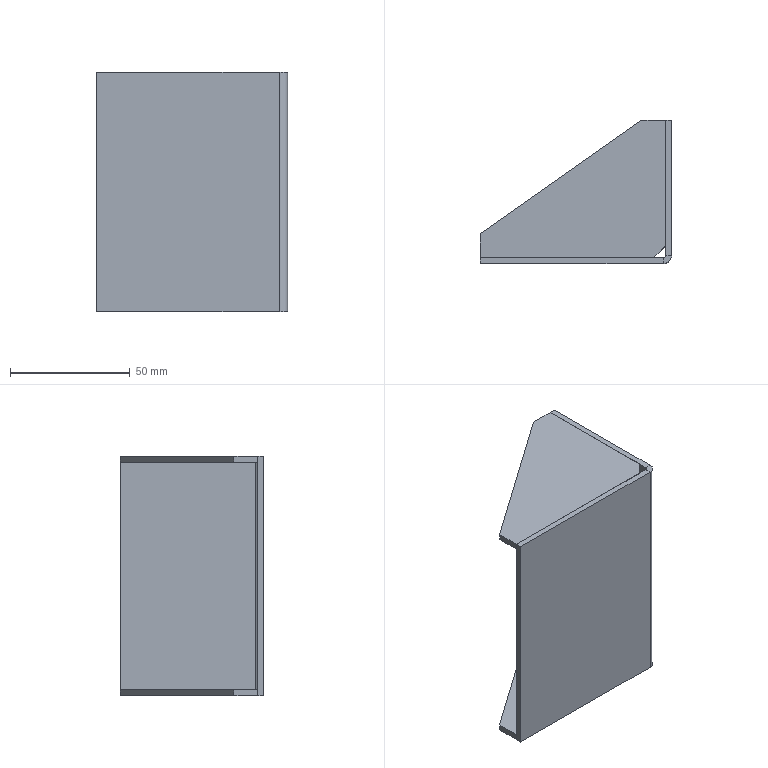Part | SolidWorks | features BaseBody 3 | 3 solids | 30 faces | box 80 x 60 x 100 mm | volume 48337 mm3 | plane 28 | cylinder 2 | commonest cylinder face diameters 2 x1 7 x1
STEP:
#1=CARTESIAN_POINT('',(-3.5,-57.5,-50.));
#2=VERTEX_POINT('',#1);
#3=CARTESIAN_POINT('',(-80.,-57.5,-50.));
#4=VERTEX_POINT('',#3);
#5=CARTESIAN_POINT('',(0.,-57.5,-50.));
#6=DIRECTION('',(-1.,0.,0.));
#7=VECTOR('',#6,1000.);
#8=LINE('',#5,#7);
#9=EDGE_CURVE('',#2,#4,#8,.T.);
#10=ORIENTED_EDGE('',*,*,#9,.F.);
#11=CARTESIAN_POINT('',(-3.5,-60.,-50.));
#12=VERTEX_POINT('',#11);
#13=CARTESIAN_POINT('',(-3.5,-57.5,-50.));
#14=DIRECTION('',(0.,-1.,0.));
#15=VECTOR('',#14,1000.);
#16=LINE('',#13,#15);
#17=EDGE_CURVE('',#2,#12,#16,.T.);
#18=ORIENTED_EDGE('',*,*,#17,.T.);
#19=CARTESIAN_POINT('',(-80.,-60.,-50.));
#20=VERTEX_POINT('',#19);
#21=CARTESIAN_POINT('',(0.,-60.,-50.));
#22=DIRECTION('',(-1.,0.,0.));
#23=VECTOR('',#22,1000.);
#24=LINE('',#21,#23);
#25=EDGE_CURVE('',#12,#20,#24,.T.);
#26=ORIENTED_EDGE('',*,*,#25,.T.);
#27=CARTESIAN_POINT('',(-80.,-60.,-50.));
#28=DIRECTION('',(0.,1.,0.));
#29=VECTOR('',#28,1000.);
#30=LINE('',#27,#29);
#31=EDGE_CURVE('',#20,#4,#30,.T.);
#32=ORIENTED_EDGE('',*,*,#31,.T.);
#33=EDGE_LOOP('',(#10,#18,#26,#32));
#34=FACE_OUTER_BOUND('',#33,.T.);
#35=CARTESIAN_POINT('',(-3.5,-56.5,-50.));
#36=DIRECTION('',(0.,0.,1.));
#37=DIRECTION('',(1.,0.,0.));
#38=AXIS2_PLACEMENT_3D('',#35,#36,#37);
#39=PLANE('',#38);
#40=ADVANCED_FACE('',(#34),#39,.F.);
#41=CARTESIAN_POINT('',(-2.5,0.,50.));
#42=VERTEX_POINT('',#41);
#43=CARTESIAN_POINT('',(-2.5,-56.5,50.));
#44=VERTEX_POINT('',#43);
#45=CARTESIAN_POINT('',(-2.5,0.,50.));
#46=DIRECTION('',(0.,-1.,0.));
#47=VECTOR('',#46,1000.);
#48=LINE('',#45,#47);
#49=EDGE_CURVE('',#42,#44,#48,.T.);
#50=ORIENTED_EDGE('',*,*,#49,.T.);
#51=CARTESIAN_POINT('',(0.,-56.5,50.));
#52=VERTEX_POINT('',#51);
#53=CARTESIAN_POINT('',(-2.5,-56.5,50.));
#54=DIRECTION('',(1.,0.,0.));
#55=VECTOR('',#54,1000.);
#56=LINE('',#53,#55);
#57=EDGE_CURVE('',#44,#52,#56,.T.);
#58=ORIENTED_EDGE('',*,*,#57,.T.);
#59=CARTESIAN_POINT('',(0.,0.,50.));
#60=VERTEX_POINT('',#59);
#61=CARTESIAN_POINT('',(0.,0.,50.));
#62=DIRECTION('',(0.,-1.,0.));
#63=VECTOR('',#62,1000.);
#64=LINE('',#61,#63);
#65=EDGE_CURVE('',#60,#52,#64,.T.);
#66=ORIENTED_EDGE('',*,*,#65,.F.);
#67=CARTESIAN_POINT('',(-2.5,0.,50.));
#68=DIRECTION('',(1.,0.,0.));
#69=VECTOR('',#68,1000.);
#70=LINE('',#67,#69);
#71=EDGE_CURVE('',#42,#60,#70,.T.);
#72=ORIENTED_EDGE('',*,*,#71,.F.);
#73=EDGE_LOOP('',(#50,#58,#66,#72));
#74=FACE_OUTER_BOUND('',#73,.T.);
#75=CARTESIAN_POINT('',(-3.5,-56.5,50.));
#76=DIRECTION('',(0.,0.,1.));
#77=DIRECTION('',(1.,0.,0.));
#78=AXIS2_PLACEMENT_3D('',#75,#76,#77);
#79=PLANE('',#78);
#80=ADVANCED_FACE('',(#74),#79,.T.);
#81=CARTESIAN_POINT('',(-2.5,-56.5,-50.));
#82=VERTEX_POINT('',#81);
#83=CARTESIAN_POINT('',(-3.5,-56.5,-50.));
#84=DIRECTION('',(0.,0.,-1.));
#85=DIRECTION('',(1.,0.,0.));
#86=AXIS2_PLACEMENT_3D('',#83,#84,#85);
#87=CIRCLE('',#86,1.);
#88=EDGE_CURVE('',#82,#2,#87,.T.);
#89=ORIENTED_EDGE('',*,*,#88,.T.);
#90=CARTESIAN_POINT('',(-3.5,-57.5,50.));
#91=VERTEX_POINT('',#90);
#92=CARTESIAN_POINT('',(-3.5,-57.5,50.));
#93=DIRECTION('',(0.,0.,-1.));
#94=VECTOR('',#93,1000.);
#95=LINE('',#92,#94);
#96=EDGE_CURVE('',#91,#2,#95,.T.);
#97=ORIENTED_EDGE('',*,*,#96,.F.);
#98=CARTESIAN_POINT('',(-3.5,-56.5,50.));
#99=DIRECTION('',(0.,0.,-1.));
#100=DIRECTION('',(1.,0.,0.));
#101=AXIS2_PLACEMENT_3D('',#98,#99,#100);
#102=CIRCLE('',#101,1.);
#103=EDGE_CURVE('',#44,#91,#102,.T.);
#104=ORIENTED_EDGE('',*,*,#103,.F.);
#105=CARTESIAN_POINT('',(-2.5,-56.5,50.));
#106=DIRECTION('',(0.,0.,-1.));
#107=VECTOR('',#106,1000.);
#108=LINE('',#105,#107);
#109=EDGE_CURVE('',#44,#82,#108,.T.);
#110=ORIENTED_EDGE('',*,*,#109,.T.);
#111=EDGE_LOOP('',(#89,#97,#104,#110));
#112=FACE_OUTER_BOUND('',#111,.T.);
#113=CARTESIAN_POINT('',(-3.5,-56.5,50.));
#114=DIRECTION('',(0.,0.,-1.));
#115=DIRECTION('',(-1.,0.,0.));
#116=AXIS2_PLACEMENT_3D('',#113,#114,#115);
#117=CYLINDRICAL_SURFACE('',#116,1.);
#118=ADVANCED_FACE('',(#112),#117,.F.);
#119=CARTESIAN_POINT('',(-2.5,0.,-50.));
#120=VERTEX_POINT('',#119);
#121=CARTESIAN_POINT('',(-2.5,0.,-50.));
#122=DIRECTION('',(0.,-1.,0.));
#123=VECTOR('',#122,1000.);
#124=LINE('',#121,#123);
#125=EDGE_CURVE('',#120,#82,#124,.T.);
#126=ORIENTED_EDGE('',*,*,#125,.T.);
#127=ORIENTED_EDGE('',*,*,#109,.F.);
#128=ORIENTED_EDGE('',*,*,#49,.F.);
#129=CARTESIAN_POINT('',(-2.5,0.,50.));
#130=DIRECTION('',(0.,0.,-1.));
#131=VECTOR('',#130,1000.);
#132=LINE('',#129,#131);
#133=EDGE_CURVE('',#42,#120,#132,.T.);
#134=ORIENTED_EDGE('',*,*,#133,.T.);
#135=EDGE_LOOP('',(#126,#127,#128,#134));
#136=FACE_OUTER_BOUND('',#135,.T.);
#137=CARTESIAN_POINT('',(-2.5,0.,50.));
#138=DIRECTION('',(1.,0.,0.));
#139=DIRECTION('',(0.,1.,0.));
#140=AXIS2_PLACEMENT_3D('',#137,#138,#139);
#141=PLANE('',#140);
#142=ADVANCED_FACE('',(#136),#141,.F.);
#143=CARTESIAN_POINT('',(0.,0.,-50.));
#144=VERTEX_POINT('',#143);
#145=CARTESIAN_POINT('',(-2.5,0.,-50.));
#146=DIRECTION('',(1.,0.,0.));
#147=VECTOR('',#146,1000.);
#148=LINE('',#145,#147);
#149=EDGE_CURVE('',#120,#144,#148,.T.);
#150=ORIENTED_EDGE('',*,*,#149,.F.);
#151=ORIENTED_EDGE('',*,*,#133,.F.);
#152=ORIENTED_EDGE('',*,*,#71,.T.);
#153=CARTESIAN_POINT('',(0.,0.,50.));
#154=DIRECTION('',(0.,0.,-1.));
#155=VECTOR('',#154,1000.);
#156=LINE('',#153,#155);
#157=EDGE_CURVE('',#60,#144,#156,.T.);
#158=ORIENTED_EDGE('',*,*,#157,.T.);
#159=EDGE_LOOP('',(#150,#151,#152,#158));
#160=FACE_OUTER_BOUND('',#159,.T.);
#161=CARTESIAN_POINT('',(-2.5,0.,50.));
#162=DIRECTION('',(0.,1.,0.));
#163=DIRECTION('',(1.,0.,0.));
#164=AXIS2_PLACEMENT_3D('',#161,#162,#163);
#165=PLANE('',#164);
#166=ADVANCED_FACE('',(#160),#165,.T.);
#167=CARTESIAN_POINT('',(0.,-56.5,-50.));
#168=VERTEX_POINT('',#167);
#169=CARTESIAN_POINT('',(0.,0.,-50.));
#170=DIRECTION('',(0.,-1.,0.));
#171=VECTOR('',#170,1000.);
#172=LINE('',#169,#171);
#173=EDGE_CURVE('',#144,#168,#172,.T.);
#174=ORIENTED_EDGE('',*,*,#173,.F.);
#175=ORIENTED_EDGE('',*,*,#157,.F.);
#176=ORIENTED_EDGE('',*,*,#65,.T.);
#177=CARTESIAN_POINT('',(0.,-56.5,50.));
#178=DIRECTION('',(0.,0.,-1.));
#179=VECTOR('',#178,1000.);
#180=LINE('',#177,#179);
#181=EDGE_CURVE('',#52,#168,#180,.T.);
#182=ORIENTED_EDGE('',*,*,#181,.T.);
#183=EDGE_LOOP('',(#174,#175,#176,#182));
#184=FACE_OUTER_BOUND('',#183,.T.);
#185=CARTESIAN_POINT('',(0.,0.,50.));
#186=DIRECTION('',(1.,0.,0.));
#187=DIRECTION('',(0.,1.,0.));
#188=AXIS2_PLACEMENT_3D('',#185,#186,#187);
#189=PLANE('',#188);
#190=ADVANCED_FACE('',(#184),#189,.T.);
#191=CARTESIAN_POINT('',(-3.5,-56.5,-50.));
#192=DIRECTION('',(0.,0.,-1.));
#193=DIRECTION('',(1.,0.,0.));
#194=AXIS2_PLACEMENT_3D('',#191,#192,#193);
#195=CIRCLE('',#194,3.5);
#196=EDGE_CURVE('',#168,#12,#195,.T.);
#197=ORIENTED_EDGE('',*,*,#196,.F.);
#198=ORIENTED_EDGE('',*,*,#181,.F.);
#199=CARTESIAN_POINT('',(-3.5,-60.,50.));
#200=VERTEX_POINT('',#199);
#201=CARTESIAN_POINT('',(-3.5,-56.5,50.));
#202=DIRECTION('',(0.,0.,-1.));
#203=DIRECTION('',(1.,0.,0.));
#204=AXIS2_PLACEMENT_3D('',#201,#202,#203);
#205=CIRCLE('',#204,3.5);
#206=EDGE_CURVE('',#52,#200,#205,.T.);
#207=ORIENTED_EDGE('',*,*,#206,.T.);
#208=CARTESIAN_POINT('',(-3.5,-60.,50.));
#209=DIRECTION('',(0.,0.,-1.));
#210=VECTOR('',#209,1000.);
#211=LINE('',#208,#210);
#212=EDGE_CURVE('',#200,#12,#211,.T.);
#213=ORIENTED_EDGE('',*,*,#212,.T.);
#214=EDGE_LOOP('',(#197,#198,#207,#213));
#215=FACE_OUTER_BOUND('',#214,.T.);
#216=CARTESIAN_POINT('',(-3.5,-56.5,50.));
#217=DIRECTION('',(0.,0.,-1.));
#218=DIRECTION('',(-1.,0.,0.));
#219=AXIS2_PLACEMENT_3D('',#216,#217,#218);
#220=CYLINDRICAL_SURFACE('',#219,3.5);
#221=ADVANCED_FACE('',(#215),#220,.T.);
#222=ORIENTED_EDGE('',*,*,#25,.F.);
#223=ORIENTED_EDGE('',*,*,#212,.F.);
#224=CARTESIAN_POINT('',(-80.,-60.,50.));
#225=VERTEX_POINT('',#224);
#226=CARTESIAN_POINT('',(0.,-60.,50.));
#227=DIRECTION('',(-1.,0.,0.));
#228=VECTOR('',#227,1000.);
#229=LINE('',#226,#228);
#230=EDGE_CURVE('',#200,#225,#229,.T.);
#231=ORIENTED_EDGE('',*,*,#230,.T.);
#232=CARTESIAN_POINT('',(-80.,-60.,50.));
#233=DIRECTION('',(0.,0.,-1.));
#234=VECTOR('',#233,1000.);
#235=LINE('',#232,#234);
#236=EDGE_CURVE('',#225,#20,#235,.T.);
#237=ORIENTED_EDGE('',*,*,#236,.T.);
#238=EDGE_LOOP('',(#222,#223,#231,#237));
#239=FACE_OUTER_BOUND('',#238,.T.);
#240=CARTESIAN_POINT('',(0.,-60.,50.));
#241=DIRECTION('',(0.,-1.,0.));
#242=DIRECTION('',(0.,0.,-1.));
#243=AXIS2_PLACEMENT_3D('',#240,#241,#242);
#244=PLANE('',#243);
#245=ADVANCED_FACE('',(#239),#244,.T.);
#246=ORIENTED_EDGE('',*,*,#31,.F.);
#247=ORIENTED_EDGE('',*,*,#236,.F.);
#248=CARTESIAN_POINT('',(-80.,-57.5,50.));
#249=VERTEX_POINT('',#248);
#250=CARTESIAN_POINT('',(-80.,-60.,50.));
#251=DIRECTION('',(0.,1.,0.));
#252=VECTOR('',#251,1000.);
#253=LINE('',#250,#252);
#254=EDGE_CURVE('',#225,#249,#253,.T.);
#255=ORIENTED_EDGE('',*,*,#254,.T.);
#256=CARTESIAN_POINT('',(-80.,-57.5,50.));
#257=DIRECTION('',(0.,0.,-1.));
#258=VECTOR('',#257,1000.);
#259=LINE('',#256,#258);
#260=EDGE_CURVE('',#249,#4,#259,.T.);
#261=ORIENTED_EDGE('',*,*,#260,.T.);
#262=EDGE_LOOP('',(#246,#247,#255,#261));
#263=FACE_OUTER_BOUND('',#262,.T.);
#264=CARTESIAN_POINT('',(-80.,-60.,50.));
#265=DIRECTION('',(-1.,0.,0.));
#266=DIRECTION('',(0.,0.,1.));
#267=AXIS2_PLACEMENT_3D('',#264,#265,#266);
#268=PLANE('',#267);
#269=ADVANCED_FACE('',(#263),#268,.T.);
#270=ORIENTED_EDGE('',*,*,#9,.T.);
#271=ORIENTED_EDGE('',*,*,#260,.F.);
#272=CARTESIAN_POINT('',(0.,-57.5,50.));
#273=DIRECTION('',(-1.,0.,0.));
#274=VECTOR('',#273,1000.);
#275=LINE('',#272,#274);
#276=EDGE_CURVE('',#91,#249,#275,.T.);
#277=ORIENTED_EDGE('',*,*,#276,.F.);
#278=ORIENTED_EDGE('',*,*,#96,.T.);
#279=EDGE_LOOP('',(#270,#271,#277,#278));
#280=FACE_OUTER_BOUND('',#279,.T.);
#281=CARTESIAN_POINT('',(0.,-57.5,50.));
#282=DIRECTION('',(0.,-1.,0.));
#283=DIRECTION('',(0.,0.,-1.));
#284=AXIS2_PLACEMENT_3D('',#281,#282,#283);
#285=PLANE('',#284);
#286=ADVANCED_FACE('',(#280),#285,.F.);
#287=ORIENTED_EDGE('',*,*,#173,.T.);
#288=CARTESIAN_POINT('',(0.,-56.5,-50.));
#289=DIRECTION('',(-1.,0.,0.));
#290=VECTOR('',#289,1000.);
#291=LINE('',#288,#290);
#292=EDGE_CURVE('',#168,#82,#291,.T.);
#293=ORIENTED_EDGE('',*,*,#292,.T.);
#294=ORIENTED_EDGE('',*,*,#125,.F.);
#295=ORIENTED_EDGE('',*,*,#149,.T.);
#296=EDGE_LOOP('',(#287,#293,#294,#295));
#297=FACE_OUTER_BOUND('',#296,.T.);
#298=CARTESIAN_POINT('',(-3.5,-57.5,-50.));
#299=DIRECTION('',(0.,0.,-1.));
#300=DIRECTION('',(0.,-1.,0.));
#301=AXIS2_PLACEMENT_3D('',#298,#299,#300);
#302=PLANE('',#301);
#303=ADVANCED_FACE('',(#297),#302,.T.);
#304=ORIENTED_EDGE('',*,*,#292,.F.);
#305=ORIENTED_EDGE('',*,*,#196,.T.);
#306=ORIENTED_EDGE('',*,*,#17,.F.);
#307=ORIENTED_EDGE('',*,*,#88,.F.);
#308=EDGE_LOOP('',(#304,#305,#306,#307));
#309=FACE_OUTER_BOUND('',#308,.T.);
#310=CARTESIAN_POINT('',(0.,-56.5,-50.));
#311=DIRECTION('',(0.,0.,-1.));
#312=DIRECTION('',(0.,-1.,0.));
#313=AXIS2_PLACEMENT_3D('',#310,#311,#312);
#314=PLANE('',#313);
#315=ADVANCED_FACE('',(#309),#314,.T.);
#316=ORIENTED_EDGE('',*,*,#230,.F.);
#317=CARTESIAN_POINT('',(-3.5,-60.,50.));
#318=DIRECTION('',(0.,1.,0.));
#319=VECTOR('',#318,1000.);
#320=LINE('',#317,#319);
#321=EDGE_CURVE('',#200,#91,#320,.T.);
#322=ORIENTED_EDGE('',*,*,#321,.T.);
#323=ORIENTED_EDGE('',*,*,#276,.T.);
#324=ORIENTED_EDGE('',*,*,#254,.F.);
#325=EDGE_LOOP('',(#316,#322,#323,#324));
#326=FACE_OUTER_BOUND('',#325,.T.);
#327=CARTESIAN_POINT('',(-2.5,-56.5,50.));
#328=DIRECTION('',(0.,0.,1.));
#329=DIRECTION('',(1.,0.,0.));
#330=AXIS2_PLACEMENT_3D('',#327,#328,#329);
#331=PLANE('',#330);
#332=ADVANCED_FACE('',(#326),#331,.T.);
#333=ORIENTED_EDGE('',*,*,#321,.F.);
#334=ORIENTED_EDGE('',*,*,#206,.F.);
#335=ORIENTED_EDGE('',*,*,#57,.F.);
#336=ORIENTED_EDGE('',*,*,#103,.T.);
#337=EDGE_LOOP('',(#333,#334,#335,#336));
#338=FACE_OUTER_BOUND('',#337,.T.);
#339=CARTESIAN_POINT('',(-3.5,-60.,50.));
#340=DIRECTION('',(0.,0.,1.));
#341=DIRECTION('',(1.,0.,0.));
#342=AXIS2_PLACEMENT_3D('',#339,#340,#341);
#343=PLANE('',#342);
#344=ADVANCED_FACE('',(#338),#343,.T.);
#345=CLOSED_SHELL('',(#40,#80,#118,#142,#166,#190,#221,#245,#269,#286,#303,#315,#332,#344));
#346=MANIFOLD_SOLID_BREP('',#345);
#347=CARTESIAN_POINT('',(-2.5,0.,-50.));
#348=VERTEX_POINT('',#347);
#349=CARTESIAN_POINT('',(-2.5,-52.5,-50.));
#350=VERTEX_POINT('',#349);
#351=CARTESIAN_POINT('',(-2.5,-52.5,-50.));
#352=DIRECTION('',(0.,-1.,0.));
#353=VECTOR('',#352,1000.);
#354=LINE('',#351,#353);
#355=EDGE_CURVE('',#348,#350,#354,.T.);
#356=ORIENTED_EDGE('',*,*,#355,.T.);
#357=CARTESIAN_POINT('',(-7.5,-57.5,-50.));
#358=VERTEX_POINT('',#357);
#359=CARTESIAN_POINT('',(-7.5,-57.5,-50.));
#360=DIRECTION('',(-0.7071,-0.7071,0.));
#361=VECTOR('',#360,1000.);
#362=LINE('',#359,#361);
#363=EDGE_CURVE('',#350,#358,#362,.T.);
#364=ORIENTED_EDGE('',*,*,#363,.T.);
#365=CARTESIAN_POINT('',(-80.,-57.5,-50.));
#366=VERTEX_POINT('',#365);
#367=CARTESIAN_POINT('',(-80.,-57.5,-50.));
#368=DIRECTION('',(-1.,0.,0.));
#369=VECTOR('',#368,1000.);
#370=LINE('',#367,#369);
#371=EDGE_CURVE('',#358,#366,#370,.T.);
#372=ORIENTED_EDGE('',*,*,#371,.T.);
#373=CARTESIAN_POINT('',(-80.,-47.5,-50.));
#374=VERTEX_POINT('',#373);
#375=CARTESIAN_POINT('',(-80.,-47.5,-50.));
#376=DIRECTION('',(0.,1.,0.));
#377=VECTOR('',#376,1000.);
#378=LINE('',#375,#377);
#379=EDGE_CURVE('',#366,#374,#378,.T.);
#380=ORIENTED_EDGE('',*,*,#379,.T.);
#381=CARTESIAN_POINT('',(-12.5,0.,-50.));
#382=VERTEX_POINT('',#381);
#383=CARTESIAN_POINT('',(-12.5,0.,-50.));
#384=DIRECTION('',(0.8178,0.5755,0.));
#385=VECTOR('',#384,1000.);
#386=LINE('',#383,#385);
#387=EDGE_CURVE('',#374,#382,#386,.T.);
#388=ORIENTED_EDGE('',*,*,#387,.T.);
#389=CARTESIAN_POINT('',(-2.5,0.,-50.));
#390=DIRECTION('',(1.,0.,0.));
#391=VECTOR('',#390,1000.);
#392=LINE('',#389,#391);
#393=EDGE_CURVE('',#382,#348,#392,.T.);
#394=ORIENTED_EDGE('',*,*,#393,.T.);
#395=EDGE_LOOP('',(#356,#364,#372,#380,#388,#394));
#396=FACE_OUTER_BOUND('',#395,.T.);
#397=CARTESIAN_POINT('',(0.,0.,-50.));
#398=DIRECTION('',(0.,0.,1.));
#399=DIRECTION('',(1.,0.,0.));
#400=AXIS2_PLACEMENT_3D('',#397,#398,#399);
#401=PLANE('',#400);
#402=ADVANCED_FACE('',(#396),#401,.F.);
#403=CARTESIAN_POINT('',(-2.5,0.,-47.5));
#404=VERTEX_POINT('',#403);
#405=CARTESIAN_POINT('',(-2.5,-52.5,-47.5));
#406=VERTEX_POINT('',#405);
#407=CARTESIAN_POINT('',(-2.5,-52.5,-47.5));
#408=DIRECTION('',(0.,-1.,0.));
#409=VECTOR('',#408,1000.);
#410=LINE('',#407,#409);
#411=EDGE_CURVE('',#404,#406,#410,.T.);
#412=ORIENTED_EDGE('',*,*,#411,.F.);
#413=CARTESIAN_POINT('',(-12.5,0.,-47.5));
#414=VERTEX_POINT('',#413);
#415=CARTESIAN_POINT('',(-2.5,0.,-47.5));
#416=DIRECTION('',(1.,0.,0.));
#417=VECTOR('',#416,1000.);
#418=LINE('',#415,#417);
#419=EDGE_CURVE('',#414,#404,#418,.T.);
#420=ORIENTED_EDGE('',*,*,#419,.F.);
#421=CARTESIAN_POINT('',(-80.,-47.5,-47.5));
#422=VERTEX_POINT('',#421);
#423=CARTESIAN_POINT('',(-12.5,0.,-47.5));
#424=DIRECTION('',(0.8178,0.5755,0.));
#425=VECTOR('',#424,1000.);
#426=LINE('',#423,#425);
#427=EDGE_CURVE('',#422,#414,#426,.T.);
#428=ORIENTED_EDGE('',*,*,#427,.F.);
#429=CARTESIAN_POINT('',(-80.,-57.5,-47.5));
#430=VERTEX_POINT('',#429);
#431=CARTESIAN_POINT('',(-80.,-47.5,-47.5));
#432=DIRECTION('',(0.,1.,0.));
#433=VECTOR('',#432,1000.);
#434=LINE('',#431,#433);
#435=EDGE_CURVE('',#430,#422,#434,.T.);
#436=ORIENTED_EDGE('',*,*,#435,.F.);
#437=CARTESIAN_POINT('',(-7.5,-57.5,-47.5));
#438=VERTEX_POINT('',#437);
#439=CARTESIAN_POINT('',(-80.,-57.5,-47.5));
#440=DIRECTION('',(-1.,0.,0.));
#441=VECTOR('',#440,1000.);
#442=LINE('',#439,#441);
#443=EDGE_CURVE('',#438,#430,#442,.T.);
#444=ORIENTED_EDGE('',*,*,#443,.F.);
#445=CARTESIAN_POINT('',(-7.5,-57.5,-47.5));
#446=DIRECTION('',(-0.7071,-0.7071,0.));
#447=VECTOR('',#446,1000.);
#448=LINE('',#445,#447);
#449=EDGE_CURVE('',#406,#438,#448,.T.);
#450=ORIENTED_EDGE('',*,*,#449,.F.);
#451=EDGE_LOOP('',(#412,#420,#428,#436,#444,#450));
#452=FACE_OUTER_BOUND('',#451,.T.);
#453=CARTESIAN_POINT('',(0.,0.,-47.5));
#454=DIRECTION('',(0.,0.,1.));
#455=DIRECTION('',(1.,0.,0.));
#456=AXIS2_PLACEMENT_3D('',#453,#454,#455);
#457=PLANE('',#456);
#458=ADVANCED_FACE('',(#452),#457,.T.);
#459=ORIENTED_EDGE('',*,*,#363,.F.);
#460=CARTESIAN_POINT('',(-2.5,-52.5,-47.5));
#461=DIRECTION('',(0.,0.,-1.));
#462=VECTOR('',#461,1000.);
#463=LINE('',#460,#462);
#464=EDGE_CURVE('',#406,#350,#463,.T.);
#465=ORIENTED_EDGE('',*,*,#464,.F.);
#466=ORIENTED_EDGE('',*,*,#449,.T.);
#467=CARTESIAN_POINT('',(-7.5,-57.5,-47.5));
#468=DIRECTION('',(0.,0.,-1.));
#469=VECTOR('',#468,1000.);
#470=LINE('',#467,#469);
#471=EDGE_CURVE('',#438,#358,#470,.T.);
#472=ORIENTED_EDGE('',*,*,#471,.T.);
#473=EDGE_LOOP('',(#459,#465,#466,#472));
#474=FACE_OUTER_BOUND('',#473,.T.);
#475=CARTESIAN_POINT('',(-7.5,-57.5,-47.5));
#476=DIRECTION('',(0.7071,-0.7071,0.));
#477=DIRECTION('',(0.,0.,-1.));
#478=AXIS2_PLACEMENT_3D('',#475,#476,#477);
#479=PLANE('',#478);
#480=ADVANCED_FACE('',(#474),#479,.T.);
#481=ORIENTED_EDGE('',*,*,#371,.F.);
#482=ORIENTED_EDGE('',*,*,#471,.F.);
#483=ORIENTED_EDGE('',*,*,#443,.T.);
#484=CARTESIAN_POINT('',(-80.,-57.5,-47.5));
#485=DIRECTION('',(0.,0.,-1.));
#486=VECTOR('',#485,1000.);
#487=LINE('',#484,#486);
#488=EDGE_CURVE('',#430,#366,#487,.T.);
#489=ORIENTED_EDGE('',*,*,#488,.T.);
#490=EDGE_LOOP('',(#481,#482,#483,#489));
#491=FACE_OUTER_BOUND('',#490,.T.);
#492=CARTESIAN_POINT('',(-80.,-57.5,-47.5));
#493=DIRECTION('',(0.,-1.,0.));
#494=DIRECTION('',(-1.,0.,0.));
#495=AXIS2_PLACEMENT_3D('',#492,#493,#494);
#496=PLANE('',#495);
#497=ADVANCED_FACE('',(#491),#496,.T.);
#498=ORIENTED_EDGE('',*,*,#379,.F.);
#499=ORIENTED_EDGE('',*,*,#488,.F.);
#500=ORIENTED_EDGE('',*,*,#435,.T.);
#501=CARTESIAN_POINT('',(-80.,-47.5,-47.5));
#502=DIRECTION('',(0.,0.,-1.));
#503=VECTOR('',#502,1000.);
#504=LINE('',#501,#503);
#505=EDGE_CURVE('',#422,#374,#504,.T.);
#506=ORIENTED_EDGE('',*,*,#505,.T.);
#507=EDGE_LOOP('',(#498,#499,#500,#506));
#508=FACE_OUTER_BOUND('',#507,.T.);
#509=CARTESIAN_POINT('',(-80.,-47.5,-47.5));
#510=DIRECTION('',(-1.,0.,0.));
#511=DIRECTION('',(0.,0.,1.));
#512=AXIS2_PLACEMENT_3D('',#509,#510,#511);
#513=PLANE('',#512);
#514=ADVANCED_FACE('',(#508),#513,.T.);
#515=ORIENTED_EDGE('',*,*,#387,.F.);
#516=ORIENTED_EDGE('',*,*,#505,.F.);
#517=ORIENTED_EDGE('',*,*,#427,.T.);
#518=CARTESIAN_POINT('',(-12.5,0.,-47.5));
#519=DIRECTION('',(0.,0.,-1.));
#520=VECTOR('',#519,1000.);
#521=LINE('',#518,#520);
#522=EDGE_CURVE('',#414,#382,#521,.T.);
#523=ORIENTED_EDGE('',*,*,#522,.T.);
#524=EDGE_LOOP('',(#515,#516,#517,#523));
#525=FACE_OUTER_BOUND('',#524,.T.);
#526=CARTESIAN_POINT('',(-12.5,0.,-47.5));
#527=DIRECTION('',(-0.5755,0.8178,0.));
#528=DIRECTION('',(0.,0.,1.));
#529=AXIS2_PLACEMENT_3D('',#526,#527,#528);
#530=PLANE('',#529);
#531=ADVANCED_FACE('',(#525),#530,.T.);
#532=ORIENTED_EDGE('',*,*,#393,.F.);
#533=ORIENTED_EDGE('',*,*,#522,.F.);
#534=ORIENTED_EDGE('',*,*,#419,.T.);
#535=CARTESIAN_POINT('',(-2.5,0.,-47.5));
#536=DIRECTION('',(0.,0.,-1.));
#537=VECTOR('',#536,1000.);
#538=LINE('',#535,#537);
#539=EDGE_CURVE('',#404,#348,#538,.T.);
#540=ORIENTED_EDGE('',*,*,#539,.T.);
#541=EDGE_LOOP('',(#532,#533,#534,#540));
#542=FACE_OUTER_BOUND('',#541,.T.);
#543=CARTESIAN_POINT('',(-2.5,0.,-47.5));
#544=DIRECTION('',(0.,1.,0.));
#545=DIRECTION('',(1.,0.,0.));
#546=AXIS2_PLACEMENT_3D('',#543,#544,#545);
#547=PLANE('',#546);
#548=ADVANCED_FACE('',(#542),#547,.T.);
#549=ORIENTED_EDGE('',*,*,#355,.F.);
#550=ORIENTED_EDGE('',*,*,#539,.F.);
#551=ORIENTED_EDGE('',*,*,#411,.T.);
#552=ORIENTED_EDGE('',*,*,#464,.T.);
#553=EDGE_LOOP('',(#549,#550,#551,#552));
#554=FACE_OUTER_BOUND('',#553,.T.);
#555=CARTESIAN_POINT('',(-2.5,-52.5,-47.5));
#556=DIRECTION('',(1.,0.,0.));
#557=DIRECTION('',(0.,1.,0.));
#558=AXIS2_PLACEMENT_3D('',#555,#556,#557);
#559=PLANE('',#558);
#560=ADVANCED_FACE('',(#554),#559,.T.);
#561=CLOSED_SHELL('',(#402,#458,#480,#497,#514,#531,#548,#560));
#562=MANIFOLD_SOLID_BREP('',#561);
#563=CARTESIAN_POINT('',(-2.5,0.,50.));
#564=VERTEX_POINT('',#563);
#565=CARTESIAN_POINT('',(-2.5,-52.5,50.));
#566=VERTEX_POINT('',#565);
#567=CARTESIAN_POINT('',(-2.5,-52.5,50.));
#568=DIRECTION('',(0.,-1.,0.));
#569=VECTOR('',#568,1000.);
#570=LINE('',#567,#569);
#571=EDGE_CURVE('',#564,#566,#570,.T.);
#572=ORIENTED_EDGE('',*,*,#571,.F.);
#573=CARTESIAN_POINT('',(-12.5,0.,50.));
#574=VERTEX_POINT('',#573);
#575=CARTESIAN_POINT('',(-2.5,0.,50.));
#576=DIRECTION('',(1.,0.,0.));
#577=VECTOR('',#576,1000.);
#578=LINE('',#575,#577);
#579=EDGE_CURVE('',#574,#564,#578,.T.);
#580=ORIENTED_EDGE('',*,*,#579,.F.);
#581=CARTESIAN_POINT('',(-80.,-47.5,50.));
#582=VERTEX_POINT('',#581);
#583=CARTESIAN_POINT('',(-12.5,0.,50.));
#584=DIRECTION('',(0.8178,0.5755,0.));
#585=VECTOR('',#584,1000.);
#586=LINE('',#583,#585);
#587=EDGE_CURVE('',#582,#574,#586,.T.);
#588=ORIENTED_EDGE('',*,*,#587,.F.);
#589=CARTESIAN_POINT('',(-80.,-57.5,50.));
#590=VERTEX_POINT('',#589);
#591=CARTESIAN_POINT('',(-80.,-47.5,50.));
#592=DIRECTION('',(0.,1.,0.));
#593=VECTOR('',#592,1000.);
#594=LINE('',#591,#593);
#595=EDGE_CURVE('',#590,#582,#594,.T.);
#596=ORIENTED_EDGE('',*,*,#595,.F.);
#597=CARTESIAN_POINT('',(-7.5,-57.5,50.));
#598=VERTEX_POINT('',#597);
#599=CARTESIAN_POINT('',(-80.,-57.5,50.));
#600=DIRECTION('',(-1.,0.,0.));
#601=VECTOR('',#600,1000.);
#602=LINE('',#599,#601);
#603=EDGE_CURVE('',#598,#590,#602,.T.);
#604=ORIENTED_EDGE('',*,*,#603,.F.);
#605=CARTESIAN_POINT('',(-7.5,-57.5,50.));
#606=DIRECTION('',(-0.7071,-0.7071,0.));
#607=VECTOR('',#606,1000.);
#608=LINE('',#605,#607);
#609=EDGE_CURVE('',#566,#598,#608,.T.);
#610=ORIENTED_EDGE('',*,*,#609,.F.);
#611=EDGE_LOOP('',(#572,#580,#588,#596,#604,#610));
#612=FACE_OUTER_BOUND('',#611,.T.);
#613=CARTESIAN_POINT('',(0.,0.,50.));
#614=DIRECTION('',(0.,0.,-1.));
#615=DIRECTION('',(0.,-1.,0.));
#616=AXIS2_PLACEMENT_3D('',#613,#614,#615);
#617=PLANE('',#616);
#618=ADVANCED_FACE('',(#612),#617,.F.);
#619=CARTESIAN_POINT('',(-2.5,0.,47.5));
#620=VERTEX_POINT('',#619);
#621=CARTESIAN_POINT('',(-2.5,-52.5,47.5));
#622=VERTEX_POINT('',#621);
#623=CARTESIAN_POINT('',(-2.5,-52.5,47.5));
#624=DIRECTION('',(0.,-1.,0.));
#625=VECTOR('',#624,1000.);
#626=LINE('',#623,#625);
#627=EDGE_CURVE('',#620,#622,#626,.T.);
#628=ORIENTED_EDGE('',*,*,#627,.T.);
#629=CARTESIAN_POINT('',(-7.5,-57.5,47.5));
#630=VERTEX_POINT('',#629);
#631=CARTESIAN_POINT('',(-7.5,-57.5,47.5));
#632=DIRECTION('',(-0.7071,-0.7071,0.));
#633=VECTOR('',#632,1000.);
#634=LINE('',#631,#633);
#635=EDGE_CURVE('',#622,#630,#634,.T.);
#636=ORIENTED_EDGE('',*,*,#635,.T.);
#637=CARTESIAN_POINT('',(-80.,-57.5,47.5));
#638=VERTEX_POINT('',#637);
#639=CARTESIAN_POINT('',(-80.,-57.5,47.5));
#640=DIRECTION('',(-1.,0.,0.));
#641=VECTOR('',#640,1000.);
#642=LINE('',#639,#641);
#643=EDGE_CURVE('',#630,#638,#642,.T.);
#644=ORIENTED_EDGE('',*,*,#643,.T.);
#645=CARTESIAN_POINT('',(-80.,-47.5,47.5));
#646=VERTEX_POINT('',#645);
#647=CARTESIAN_POINT('',(-80.,-47.5,47.5));
#648=DIRECTION('',(0.,1.,0.));
#649=VECTOR('',#648,1000.);
#650=LINE('',#647,#649);
#651=EDGE_CURVE('',#638,#646,#650,.T.);
#652=ORIENTED_EDGE('',*,*,#651,.T.);
#653=CARTESIAN_POINT('',(-12.5,0.,47.5));
#654=VERTEX_POINT('',#653);
#655=CARTESIAN_POINT('',(-12.5,0.,47.5));
#656=DIRECTION('',(0.8178,0.5755,0.));
#657=VECTOR('',#656,1000.);
#658=LINE('',#655,#657);
#659=EDGE_CURVE('',#646,#654,#658,.T.);
#660=ORIENTED_EDGE('',*,*,#659,.T.);
#661=CARTESIAN_POINT('',(-2.5,0.,47.5));
#662=DIRECTION('',(1.,0.,0.));
#663=VECTOR('',#662,1000.);
#664=LINE('',#661,#663);
#665=EDGE_CURVE('',#654,#620,#664,.T.);
#666=ORIENTED_EDGE('',*,*,#665,.T.);
#667=EDGE_LOOP('',(#628,#636,#644,#652,#660,#666));
#668=FACE_OUTER_BOUND('',#667,.T.);
#669=CARTESIAN_POINT('',(0.,0.,47.5));
#670=DIRECTION('',(0.,0.,-1.));
#671=DIRECTION('',(0.,-1.,0.));
#672=AXIS2_PLACEMENT_3D('',#669,#670,#671);
#673=PLANE('',#672);
#674=ADVANCED_FACE('',(#668),#673,.T.);
#675=ORIENTED_EDGE('',*,*,#609,.T.);
#676=CARTESIAN_POINT('',(-7.5,-57.5,47.5));
#677=DIRECTION('',(0.,0.,1.));
#678=VECTOR('',#677,1000.);
#679=LINE('',#676,#678);
#680=EDGE_CURVE('',#630,#598,#679,.T.);
#681=ORIENTED_EDGE('',*,*,#680,.F.);
#682=ORIENTED_EDGE('',*,*,#635,.F.);
#683=CARTESIAN_POINT('',(-2.5,-52.5,47.5));
#684=DIRECTION('',(0.,0.,1.));
#685=VECTOR('',#684,1000.);
#686=LINE('',#683,#685);
#687=EDGE_CURVE('',#622,#566,#686,.T.);
#688=ORIENTED_EDGE('',*,*,#687,.T.);
#689=EDGE_LOOP('',(#675,#681,#682,#688));
#690=FACE_OUTER_BOUND('',#689,.T.);
#691=CARTESIAN_POINT('',(-7.5,-57.5,47.5));
#692=DIRECTION('',(0.7071,-0.7071,0.));
#693=DIRECTION('',(0.,0.,-1.));
#694=AXIS2_PLACEMENT_3D('',#691,#692,#693);
#695=PLANE('',#694);
#696=ADVANCED_FACE('',(#690),#695,.T.);
#697=ORIENTED_EDGE('',*,*,#603,.T.);
#698=CARTESIAN_POINT('',(-80.,-57.5,47.5));
#699=DIRECTION('',(0.,0.,1.));
#700=VECTOR('',#699,1000.);
#701=LINE('',#698,#700);
#702=EDGE_CURVE('',#638,#590,#701,.T.);
#703=ORIENTED_EDGE('',*,*,#702,.F.);
#704=ORIENTED_EDGE('',*,*,#643,.F.);
#705=ORIENTED_EDGE('',*,*,#680,.T.);
#706=EDGE_LOOP('',(#697,#703,#704,#705));
#707=FACE_OUTER_BOUND('',#706,.T.);
#708=CARTESIAN_POINT('',(-80.,-57.5,47.5));
#709=DIRECTION('',(0.,-1.,0.));
#710=DIRECTION('',(-1.,0.,0.));
#711=AXIS2_PLACEMENT_3D('',#708,#709,#710);
#712=PLANE('',#711);
#713=ADVANCED_FACE('',(#707),#712,.T.);
#714=ORIENTED_EDGE('',*,*,#595,.T.);
#715=CARTESIAN_POINT('',(-80.,-47.5,47.5));
#716=DIRECTION('',(0.,0.,1.));
#717=VECTOR('',#716,1000.);
#718=LINE('',#715,#717);
#719=EDGE_CURVE('',#646,#582,#718,.T.);
#720=ORIENTED_EDGE('',*,*,#719,.F.);
#721=ORIENTED_EDGE('',*,*,#651,.F.);
#722=ORIENTED_EDGE('',*,*,#702,.T.);
#723=EDGE_LOOP('',(#714,#720,#721,#722));
#724=FACE_OUTER_BOUND('',#723,.T.);
#725=CARTESIAN_POINT('',(-80.,-47.5,47.5));
#726=DIRECTION('',(-1.,0.,0.));
#727=DIRECTION('',(0.,0.,1.));
#728=AXIS2_PLACEMENT_3D('',#725,#726,#727);
#729=PLANE('',#728);
#730=ADVANCED_FACE('',(#724),#729,.T.);
#731=ORIENTED_EDGE('',*,*,#587,.T.);
#732=CARTESIAN_POINT('',(-12.5,0.,47.5));
#733=DIRECTION('',(0.,0.,1.));
#734=VECTOR('',#733,1000.);
#735=LINE('',#732,#734);
#736=EDGE_CURVE('',#654,#574,#735,.T.);
#737=ORIENTED_EDGE('',*,*,#736,.F.);
#738=ORIENTED_EDGE('',*,*,#659,.F.);
#739=ORIENTED_EDGE('',*,*,#719,.T.);
#740=EDGE_LOOP('',(#731,#737,#738,#739));
#741=FACE_OUTER_BOUND('',#740,.T.);
#742=CARTESIAN_POINT('',(-12.5,0.,47.5));
#743=DIRECTION('',(-0.5755,0.8178,0.));
#744=DIRECTION('',(0.,0.,1.));
#745=AXIS2_PLACEMENT_3D('',#742,#743,#744);
#746=PLANE('',#745);
#747=ADVANCED_FACE('',(#741),#746,.T.);
#748=ORIENTED_EDGE('',*,*,#579,.T.);
#749=CARTESIAN_POINT('',(-2.5,0.,47.5));
#750=DIRECTION('',(0.,0.,1.));
#751=VECTOR('',#750,1000.);
#752=LINE('',#749,#751);
#753=EDGE_CURVE('',#620,#564,#752,.T.);
#754=ORIENTED_EDGE('',*,*,#753,.F.);
#755=ORIENTED_EDGE('',*,*,#665,.F.);
#756=ORIENTED_EDGE('',*,*,#736,.T.);
#757=EDGE_LOOP('',(#748,#754,#755,#756));
#758=FACE_OUTER_BOUND('',#757,.T.);
#759=CARTESIAN_POINT('',(-2.5,0.,47.5));
#760=DIRECTION('',(0.,1.,0.));
#761=DIRECTION('',(1.,0.,0.));
#762=AXIS2_PLACEMENT_3D('',#759,#760,#761);
#763=PLANE('',#762);
#764=ADVANCED_FACE('',(#758),#763,.T.);
#765=ORIENTED_EDGE('',*,*,#571,.T.);
#766=ORIENTED_EDGE('',*,*,#687,.F.);
#767=ORIENTED_EDGE('',*,*,#627,.F.);
#768=ORIENTED_EDGE('',*,*,#753,.T.);
#769=EDGE_LOOP('',(#765,#766,#767,#768));
#770=FACE_OUTER_BOUND('',#769,.T.);
#771=CARTESIAN_POINT('',(-2.5,-52.5,47.5));
#772=DIRECTION('',(1.,0.,0.));
#773=DIRECTION('',(0.,1.,0.));
#774=AXIS2_PLACEMENT_3D('',#771,#772,#773);
#775=PLANE('',#774);
#776=ADVANCED_FACE('',(#770),#775,.T.);
#777=CLOSED_SHELL('',(#618,#674,#696,#713,#730,#747,#764,#776));
#778=MANIFOLD_SOLID_BREP('',#777);
#779=CARTESIAN_POINT('',(0.,0.,0.));
#780=DIRECTION('',(0.,0.,1.));
#781=DIRECTION('',(1.,0.,0.));
#782=AXIS2_PLACEMENT_3D('',#779,#780,#781);
#783=(LENGTH_UNIT()NAMED_UNIT(*)SI_UNIT(.MILLI.,.METRE.));
#784=UNCERTAINTY_MEASURE_WITH_UNIT(LENGTH_MEASURE(0.00001),#783,'','');
#785=(NAMED_UNIT(*)PLANE_ANGLE_UNIT()SI_UNIT($,.RADIAN.));
#786=(NAMED_UNIT(*)SI_UNIT($,.STERADIAN.)SOLID_ANGLE_UNIT());
#787=(GEOMETRIC_REPRESENTATION_CONTEXT(3)GLOBAL_UNCERTAINTY_ASSIGNED_CONTEXT((#784))GLOBAL_UNIT_ASSIGNED_CONTEXT((#783,#785,#786))REPRESENTATION_CONTEXT('',''));
#788=ADVANCED_BREP_SHAPE_REPRESENTATION('',(#346,#562,#778,#782),#787);